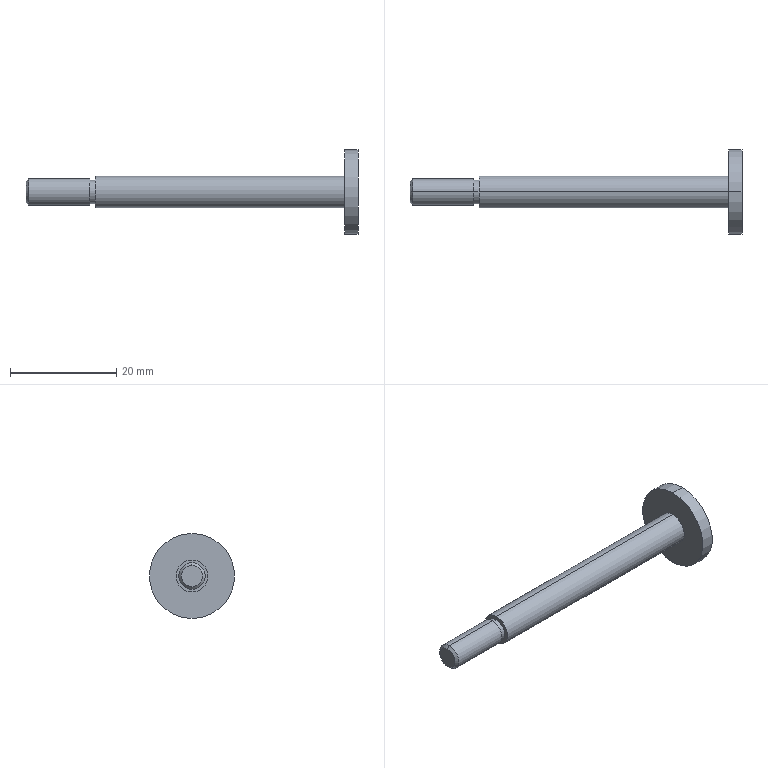Part | SolidWorks | features RefAxis 9, 3DProfileFeature 3, Revolution 3 | 1 solid | 15 faces | box 62.5 x 16 x 16 mm | volume 2081 mm3 | cylinder 8 | plane 5 | cone 2 | commonest cylinder face diameters 4.4 x2 5 x2 6 x2 16 x2
STEP:
#1=CARTESIAN_POINT('',(-23.509,0.,-2.5));
#2=VERTEX_POINT('',#1);
#3=CARTESIAN_POINT('',(-23.509,0.,2.5));
#4=VERTEX_POINT('',#3);
#5=CARTESIAN_POINT('',(-23.509,0.,0.));
#6=DIRECTION('',(1.,0.,0.));
#7=DIRECTION('',(0.,0.,-1.));
#8=AXIS2_PLACEMENT_3D('',#5,#6,#7);
#9=CIRCLE('',#8,2.5);
#10=EDGE_CURVE('',#2,#4,#9,.T.);
#11=ORIENTED_EDGE('',*,*,#10,.T.);
#12=CARTESIAN_POINT('',(-12.,0.,2.5));
#13=VERTEX_POINT('',#12);
#14=CARTESIAN_POINT('',(-12.,0.,2.5));
#15=DIRECTION('',(1.,0.,0.));
#16=VECTOR('',#15,1000.);
#17=LINE('',#14,#16);
#18=EDGE_CURVE('',#4,#13,#17,.T.);
#19=ORIENTED_EDGE('',*,*,#18,.T.);
#20=CARTESIAN_POINT('',(-12.,0.,-2.5));
#21=VERTEX_POINT('',#20);
#22=CARTESIAN_POINT('',(-12.,0.,0.));
#23=DIRECTION('',(1.,0.,0.));
#24=DIRECTION('',(0.,0.,-1.));
#25=AXIS2_PLACEMENT_3D('',#22,#23,#24);
#26=CIRCLE('',#25,2.5);
#27=EDGE_CURVE('',#21,#13,#26,.T.);
#28=ORIENTED_EDGE('',*,*,#27,.F.);
#29=CARTESIAN_POINT('',(-12.,0.,-2.5));
#30=DIRECTION('',(1.,0.,0.));
#31=VECTOR('',#30,1000.);
#32=LINE('',#29,#31);
#33=EDGE_CURVE('',#2,#21,#32,.T.);
#34=ORIENTED_EDGE('',*,*,#33,.F.);
#35=EDGE_LOOP('',(#11,#19,#28,#34));
#36=FACE_OUTER_BOUND('',#35,.T.);
#37=CARTESIAN_POINT('',(-12.,0.,0.));
#38=DIRECTION('',(1.,0.,0.));
#39=DIRECTION('',(0.,0.,-1.));
#40=AXIS2_PLACEMENT_3D('',#37,#38,#39);
#41=CYLINDRICAL_SURFACE('',#40,2.5);
#42=ADVANCED_FACE('',(#36),#41,.T.);
#43=CARTESIAN_POINT('',(-24.,0.,-2.01));
#44=VERTEX_POINT('',#43);
#45=CARTESIAN_POINT('',(-24.,0.,2.01));
#46=VERTEX_POINT('',#45);
#47=CARTESIAN_POINT('',(-24.,0.,0.));
#48=DIRECTION('',(1.,0.,0.));
#49=DIRECTION('',(0.,0.,-1.));
#50=AXIS2_PLACEMENT_3D('',#47,#48,#49);
#51=CIRCLE('',#50,2.01);
#52=EDGE_CURVE('',#44,#46,#51,.T.);
#53=ORIENTED_EDGE('',*,*,#52,.T.);
#54=CARTESIAN_POINT('',(-23.509,0.,2.5));
#55=DIRECTION('',(0.7071,0.,0.7071));
#56=VECTOR('',#55,1000.);
#57=LINE('',#54,#56);
#58=EDGE_CURVE('',#46,#4,#57,.T.);
#59=ORIENTED_EDGE('',*,*,#58,.T.);
#60=ORIENTED_EDGE('',*,*,#10,.F.);
#61=CARTESIAN_POINT('',(-23.509,0.,-2.5));
#62=DIRECTION('',(0.7071,0.,-0.7071));
#63=VECTOR('',#62,1000.);
#64=LINE('',#61,#63);
#65=EDGE_CURVE('',#44,#2,#64,.T.);
#66=ORIENTED_EDGE('',*,*,#65,.F.);
#67=EDGE_LOOP('',(#53,#59,#60,#66));
#68=FACE_OUTER_BOUND('',#67,.T.);
#69=CARTESIAN_POINT('',(-23.509,0.,0.));
#70=DIRECTION('',(1.,0.,0.));
#71=DIRECTION('',(0.,0.,-1.));
#72=AXIS2_PLACEMENT_3D('',#69,#70,#71);
#73=CONICAL_SURFACE('',#72,2.5,0.7854);
#74=ADVANCED_FACE('',(#68),#73,.T.);
#75=CARTESIAN_POINT('',(-12.,0.,2.2));
#76=VERTEX_POINT('',#75);
#77=CARTESIAN_POINT('',(-12.,0.,-2.2));
#78=VERTEX_POINT('',#77);
#79=CARTESIAN_POINT('',(-12.,0.,0.));
#80=DIRECTION('',(-1.,0.,0.));
#81=DIRECTION('',(0.,0.,-1.));
#82=AXIS2_PLACEMENT_3D('',#79,#80,#81);
#83=CIRCLE('',#82,2.2);
#84=EDGE_CURVE('',#76,#78,#83,.T.);
#85=ORIENTED_EDGE('',*,*,#84,.F.);
#86=CARTESIAN_POINT('',(-11.,0.,2.2));
#87=VERTEX_POINT('',#86);
#88=CARTESIAN_POINT('',(-11.,0.,2.2));
#89=DIRECTION('',(1.,0.,0.));
#90=VECTOR('',#89,1000.);
#91=LINE('',#88,#90);
#92=EDGE_CURVE('',#76,#87,#91,.T.);
#93=ORIENTED_EDGE('',*,*,#92,.T.);
#94=CARTESIAN_POINT('',(-11.,0.,-2.2));
#95=VERTEX_POINT('',#94);
#96=CARTESIAN_POINT('',(-11.,0.,0.));
#97=DIRECTION('',(-1.,0.,0.));
#98=DIRECTION('',(0.,0.,1.));
#99=AXIS2_PLACEMENT_3D('',#96,#97,#98);
#100=CIRCLE('',#99,2.2);
#101=EDGE_CURVE('',#87,#95,#100,.T.);
#102=ORIENTED_EDGE('',*,*,#101,.T.);
#103=CARTESIAN_POINT('',(-11.,0.,-2.2));
#104=DIRECTION('',(1.,0.,0.));
#105=VECTOR('',#104,1000.);
#106=LINE('',#103,#105);
#107=EDGE_CURVE('',#78,#95,#106,.T.);
#108=ORIENTED_EDGE('',*,*,#107,.F.);
#109=EDGE_LOOP('',(#85,#93,#102,#108));
#110=FACE_OUTER_BOUND('',#109,.T.);
#111=CARTESIAN_POINT('',(-11.,0.,0.));
#112=DIRECTION('',(1.,0.,0.));
#113=DIRECTION('',(0.,0.,-1.));
#114=AXIS2_PLACEMENT_3D('',#111,#112,#113);
#115=CYLINDRICAL_SURFACE('',#114,2.2);
#116=ADVANCED_FACE('',(#110),#115,.T.);
#117=CARTESIAN_POINT('',(36.,0.,-8.));
#118=VERTEX_POINT('',#117);
#119=CARTESIAN_POINT('',(36.,0.,8.));
#120=VERTEX_POINT('',#119);
#121=CARTESIAN_POINT('',(36.,0.,0.));
#122=DIRECTION('',(1.,0.,0.));
#123=DIRECTION('',(0.,0.,-1.));
#124=AXIS2_PLACEMENT_3D('',#121,#122,#123);
#125=CIRCLE('',#124,8.);
#126=EDGE_CURVE('',#118,#120,#125,.T.);
#127=ORIENTED_EDGE('',*,*,#126,.T.);
#128=CARTESIAN_POINT('',(38.5,0.,8.));
#129=VERTEX_POINT('',#128);
#130=CARTESIAN_POINT('',(38.5,0.,8.));
#131=DIRECTION('',(1.,0.,0.));
#132=VECTOR('',#131,1000.);
#133=LINE('',#130,#132);
#134=EDGE_CURVE('',#120,#129,#133,.T.);
#135=ORIENTED_EDGE('',*,*,#134,.T.);
#136=CARTESIAN_POINT('',(38.5,0.,-8.));
#137=VERTEX_POINT('',#136);
#138=CARTESIAN_POINT('',(38.5,0.,0.));
#139=DIRECTION('',(1.,0.,0.));
#140=DIRECTION('',(0.,0.,-1.));
#141=AXIS2_PLACEMENT_3D('',#138,#139,#140);
#142=CIRCLE('',#141,8.);
#143=EDGE_CURVE('',#137,#129,#142,.T.);
#144=ORIENTED_EDGE('',*,*,#143,.F.);
#145=CARTESIAN_POINT('',(38.5,0.,-8.));
#146=DIRECTION('',(1.,0.,0.));
#147=VECTOR('',#146,1000.);
#148=LINE('',#145,#147);
#149=EDGE_CURVE('',#118,#137,#148,.T.);
#150=ORIENTED_EDGE('',*,*,#149,.F.);
#151=EDGE_LOOP('',(#127,#135,#144,#150));
#152=FACE_OUTER_BOUND('',#151,.T.);
#153=CARTESIAN_POINT('',(38.5,0.,0.));
#154=DIRECTION('',(1.,0.,0.));
#155=DIRECTION('',(0.,0.,-1.));
#156=AXIS2_PLACEMENT_3D('',#153,#154,#155);
#157=CYLINDRICAL_SURFACE('',#156,8.);
#158=ADVANCED_FACE('',(#152),#157,.T.);
#159=CARTESIAN_POINT('',(-11.,0.,-3.));
#160=VERTEX_POINT('',#159);
#161=CARTESIAN_POINT('',(-11.,0.,3.));
#162=VERTEX_POINT('',#161);
#163=CARTESIAN_POINT('',(-11.,0.,0.));
#164=DIRECTION('',(1.,0.,0.));
#165=DIRECTION('',(0.,0.,-1.));
#166=AXIS2_PLACEMENT_3D('',#163,#164,#165);
#167=CIRCLE('',#166,3.);
#168=EDGE_CURVE('',#160,#162,#167,.T.);
#169=ORIENTED_EDGE('',*,*,#168,.T.);
#170=CARTESIAN_POINT('',(36.,0.,3.));
#171=VERTEX_POINT('',#170);
#172=CARTESIAN_POINT('',(38.5,0.,3.));
#173=DIRECTION('',(1.,0.,0.));
#174=VECTOR('',#173,1000.);
#175=LINE('',#172,#174);
#176=EDGE_CURVE('',#162,#171,#175,.T.);
#177=ORIENTED_EDGE('',*,*,#176,.T.);
#178=CARTESIAN_POINT('',(36.,0.,-3.));
#179=VERTEX_POINT('',#178);
#180=CARTESIAN_POINT('',(36.,0.,0.));
#181=DIRECTION('',(1.,0.,0.));
#182=DIRECTION('',(0.,0.,-1.));
#183=AXIS2_PLACEMENT_3D('',#180,#181,#182);
#184=CIRCLE('',#183,3.);
#185=EDGE_CURVE('',#179,#171,#184,.T.);
#186=ORIENTED_EDGE('',*,*,#185,.F.);
#187=CARTESIAN_POINT('',(38.5,0.,-3.));
#188=DIRECTION('',(1.,0.,0.));
#189=VECTOR('',#188,1000.);
#190=LINE('',#187,#189);
#191=EDGE_CURVE('',#160,#179,#190,.T.);
#192=ORIENTED_EDGE('',*,*,#191,.F.);
#193=EDGE_LOOP('',(#169,#177,#186,#192));
#194=FACE_OUTER_BOUND('',#193,.T.);
#195=CARTESIAN_POINT('',(38.5,0.,0.));
#196=DIRECTION('',(1.,0.,0.));
#197=DIRECTION('',(0.,0.,-1.));
#198=AXIS2_PLACEMENT_3D('',#195,#196,#197);
#199=CYLINDRICAL_SURFACE('',#198,3.);
#200=ADVANCED_FACE('',(#194),#199,.T.);
#201=CARTESIAN_POINT('',(-11.,0.,0.));
#202=DIRECTION('',(-1.,0.,0.));
#203=DIRECTION('',(0.,0.,1.));
#204=AXIS2_PLACEMENT_3D('',#201,#202,#203);
#205=CIRCLE('',#204,2.2);
#206=EDGE_CURVE('',#95,#87,#205,.T.);
#207=ORIENTED_EDGE('',*,*,#206,.F.);
#208=ORIENTED_EDGE('',*,*,#101,.F.);
#209=EDGE_LOOP('',(#207,#208));
#210=FACE_BOUND('',#209,.T.);
#211=ORIENTED_EDGE('',*,*,#168,.F.);
#212=CARTESIAN_POINT('',(-11.,0.,0.));
#213=DIRECTION('',(1.,0.,0.));
#214=DIRECTION('',(0.,0.,-1.));
#215=AXIS2_PLACEMENT_3D('',#212,#213,#214);
#216=CIRCLE('',#215,3.);
#217=EDGE_CURVE('',#162,#160,#216,.T.);
#218=ORIENTED_EDGE('',*,*,#217,.F.);
#219=EDGE_LOOP('',(#211,#218));
#220=FACE_OUTER_BOUND('',#219,.T.);
#221=CARTESIAN_POINT('',(-11.,0.,0.));
#222=DIRECTION('',(-1.,0.,0.));
#223=DIRECTION('',(0.,0.,1.));
#224=AXIS2_PLACEMENT_3D('',#221,#222,#223);
#225=PLANE('',#224);
#226=ADVANCED_FACE('',(#210,#220),#225,.T.);
#227=ORIENTED_EDGE('',*,*,#176,.F.);
#228=ORIENTED_EDGE('',*,*,#217,.T.);
#229=ORIENTED_EDGE('',*,*,#191,.T.);
#230=CARTESIAN_POINT('',(36.,0.,0.));
#231=DIRECTION('',(1.,0.,0.));
#232=DIRECTION('',(0.,0.,-1.));
#233=AXIS2_PLACEMENT_3D('',#230,#231,#232);
#234=CIRCLE('',#233,3.);
#235=EDGE_CURVE('',#171,#179,#234,.T.);
#236=ORIENTED_EDGE('',*,*,#235,.F.);
#237=EDGE_LOOP('',(#227,#228,#229,#236));
#238=FACE_OUTER_BOUND('',#237,.T.);
#239=CARTESIAN_POINT('',(38.5,0.,0.));
#240=DIRECTION('',(1.,0.,0.));
#241=DIRECTION('',(0.,0.,-1.));
#242=AXIS2_PLACEMENT_3D('',#239,#240,#241);
#243=CYLINDRICAL_SURFACE('',#242,3.);
#244=ADVANCED_FACE('',(#238),#243,.T.);
#245=ORIENTED_EDGE('',*,*,#185,.T.);
#246=ORIENTED_EDGE('',*,*,#235,.T.);
#247=EDGE_LOOP('',(#245,#246));
#248=FACE_BOUND('',#247,.T.);
#249=ORIENTED_EDGE('',*,*,#126,.F.);
#250=CARTESIAN_POINT('',(36.,0.,0.));
#251=DIRECTION('',(1.,0.,0.));
#252=DIRECTION('',(0.,0.,-1.));
#253=AXIS2_PLACEMENT_3D('',#250,#251,#252);
#254=CIRCLE('',#253,8.);
#255=EDGE_CURVE('',#120,#118,#254,.T.);
#256=ORIENTED_EDGE('',*,*,#255,.F.);
#257=EDGE_LOOP('',(#249,#256));
#258=FACE_OUTER_BOUND('',#257,.T.);
#259=CARTESIAN_POINT('',(36.,3.,0.));
#260=DIRECTION('',(-1.,0.,0.));
#261=DIRECTION('',(0.,0.,1.));
#262=AXIS2_PLACEMENT_3D('',#259,#260,#261);
#263=PLANE('',#262);
#264=ADVANCED_FACE('',(#248,#258),#263,.T.);
#265=ORIENTED_EDGE('',*,*,#134,.F.);
#266=ORIENTED_EDGE('',*,*,#255,.T.);
#267=ORIENTED_EDGE('',*,*,#149,.T.);
#268=CARTESIAN_POINT('',(38.5,0.,0.));
#269=DIRECTION('',(1.,0.,0.));
#270=DIRECTION('',(0.,0.,-1.));
#271=AXIS2_PLACEMENT_3D('',#268,#269,#270);
#272=CIRCLE('',#271,8.);
#273=EDGE_CURVE('',#129,#137,#272,.T.);
#274=ORIENTED_EDGE('',*,*,#273,.F.);
#275=EDGE_LOOP('',(#265,#266,#267,#274));
#276=FACE_OUTER_BOUND('',#275,.T.);
#277=CARTESIAN_POINT('',(38.5,0.,0.));
#278=DIRECTION('',(1.,0.,0.));
#279=DIRECTION('',(0.,0.,-1.));
#280=AXIS2_PLACEMENT_3D('',#277,#278,#279);
#281=CYLINDRICAL_SURFACE('',#280,8.);
#282=ADVANCED_FACE('',(#276),#281,.T.);
#283=ORIENTED_EDGE('',*,*,#143,.T.);
#284=ORIENTED_EDGE('',*,*,#273,.T.);
#285=EDGE_LOOP('',(#283,#284));
#286=FACE_OUTER_BOUND('',#285,.T.);
#287=CARTESIAN_POINT('',(38.5,8.,0.));
#288=DIRECTION('',(1.,0.,0.));
#289=DIRECTION('',(0.,0.,-1.));
#290=AXIS2_PLACEMENT_3D('',#287,#288,#289);
#291=PLANE('',#290);
#292=ADVANCED_FACE('',(#286),#291,.T.);
#293=ORIENTED_EDGE('',*,*,#92,.F.);
#294=CARTESIAN_POINT('',(-12.,0.,0.));
#295=DIRECTION('',(-1.,0.,0.));
#296=DIRECTION('',(0.,0.,-1.));
#297=AXIS2_PLACEMENT_3D('',#294,#295,#296);
#298=CIRCLE('',#297,2.2);
#299=EDGE_CURVE('',#78,#76,#298,.T.);
#300=ORIENTED_EDGE('',*,*,#299,.F.);
#301=ORIENTED_EDGE('',*,*,#107,.T.);
#302=ORIENTED_EDGE('',*,*,#206,.T.);
#303=EDGE_LOOP('',(#293,#300,#301,#302));
#304=FACE_OUTER_BOUND('',#303,.T.);
#305=CARTESIAN_POINT('',(-11.,0.,0.));
#306=DIRECTION('',(1.,0.,0.));
#307=DIRECTION('',(0.,0.,-1.));
#308=AXIS2_PLACEMENT_3D('',#305,#306,#307);
#309=CYLINDRICAL_SURFACE('',#308,2.2);
#310=ADVANCED_FACE('',(#304),#309,.T.);
#311=ORIENTED_EDGE('',*,*,#52,.F.);
#312=CARTESIAN_POINT('',(-24.,0.,0.));
#313=DIRECTION('',(1.,0.,0.));
#314=DIRECTION('',(0.,0.,-1.));
#315=AXIS2_PLACEMENT_3D('',#312,#313,#314);
#316=CIRCLE('',#315,2.01);
#317=EDGE_CURVE('',#46,#44,#316,.T.);
#318=ORIENTED_EDGE('',*,*,#317,.F.);
#319=EDGE_LOOP('',(#311,#318));
#320=FACE_OUTER_BOUND('',#319,.T.);
#321=CARTESIAN_POINT('',(-24.,0.,0.));
#322=DIRECTION('',(-1.,0.,0.));
#323=DIRECTION('',(0.,0.,1.));
#324=AXIS2_PLACEMENT_3D('',#321,#322,#323);
#325=PLANE('',#324);
#326=ADVANCED_FACE('',(#320),#325,.T.);
#327=ORIENTED_EDGE('',*,*,#58,.F.);
#328=ORIENTED_EDGE('',*,*,#317,.T.);
#329=ORIENTED_EDGE('',*,*,#65,.T.);
#330=CARTESIAN_POINT('',(-23.509,0.,0.));
#331=DIRECTION('',(1.,0.,0.));
#332=DIRECTION('',(0.,0.,-1.));
#333=AXIS2_PLACEMENT_3D('',#330,#331,#332);
#334=CIRCLE('',#333,2.5);
#335=EDGE_CURVE('',#4,#2,#334,.T.);
#336=ORIENTED_EDGE('',*,*,#335,.F.);
#337=EDGE_LOOP('',(#327,#328,#329,#336));
#338=FACE_OUTER_BOUND('',#337,.T.);
#339=CARTESIAN_POINT('',(-23.509,0.,0.));
#340=DIRECTION('',(1.,0.,0.));
#341=DIRECTION('',(0.,0.,-1.));
#342=AXIS2_PLACEMENT_3D('',#339,#340,#341);
#343=CONICAL_SURFACE('',#342,2.5,0.7854);
#344=ADVANCED_FACE('',(#338),#343,.T.);
#345=ORIENTED_EDGE('',*,*,#18,.F.);
#346=ORIENTED_EDGE('',*,*,#335,.T.);
#347=ORIENTED_EDGE('',*,*,#33,.T.);
#348=CARTESIAN_POINT('',(-12.,0.,0.));
#349=DIRECTION('',(1.,0.,0.));
#350=DIRECTION('',(0.,0.,-1.));
#351=AXIS2_PLACEMENT_3D('',#348,#349,#350);
#352=CIRCLE('',#351,2.5);
#353=EDGE_CURVE('',#13,#21,#352,.T.);
#354=ORIENTED_EDGE('',*,*,#353,.F.);
#355=EDGE_LOOP('',(#345,#346,#347,#354));
#356=FACE_OUTER_BOUND('',#355,.T.);
#357=CARTESIAN_POINT('',(-12.,0.,0.));
#358=DIRECTION('',(1.,0.,0.));
#359=DIRECTION('',(0.,0.,-1.));
#360=AXIS2_PLACEMENT_3D('',#357,#358,#359);
#361=CYLINDRICAL_SURFACE('',#360,2.5);
#362=ADVANCED_FACE('',(#356),#361,.T.);
#363=ORIENTED_EDGE('',*,*,#299,.T.);
#364=ORIENTED_EDGE('',*,*,#84,.T.);
#365=EDGE_LOOP('',(#363,#364));
#366=FACE_BOUND('',#365,.T.);
#367=ORIENTED_EDGE('',*,*,#27,.T.);
#368=ORIENTED_EDGE('',*,*,#353,.T.);
#369=EDGE_LOOP('',(#367,#368));
#370=FACE_OUTER_BOUND('',#369,.T.);
#371=CARTESIAN_POINT('',(-12.,2.5,0.));
#372=DIRECTION('',(1.,0.,0.));
#373=DIRECTION('',(0.,0.,-1.));
#374=AXIS2_PLACEMENT_3D('',#371,#372,#373);
#375=PLANE('',#374);
#376=ADVANCED_FACE('',(#366,#370),#375,.T.);
#377=CLOSED_SHELL('',(#42,#74,#116,#158,#200,#226,#244,#264,#282,#292,#310,#326,#344,#362,#376));
#378=MANIFOLD_SOLID_BREP('',#377);
#379=CARTESIAN_POINT('',(0.,0.,0.));
#380=DIRECTION('',(0.,0.,1.));
#381=DIRECTION('',(1.,0.,0.));
#382=AXIS2_PLACEMENT_3D('',#379,#380,#381);
#383=(LENGTH_UNIT()NAMED_UNIT(*)SI_UNIT(.MILLI.,.METRE.));
#384=UNCERTAINTY_MEASURE_WITH_UNIT(LENGTH_MEASURE(0.00001),#383,'','');
#385=(NAMED_UNIT(*)PLANE_ANGLE_UNIT()SI_UNIT($,.RADIAN.));
#386=(NAMED_UNIT(*)SI_UNIT($,.STERADIAN.)SOLID_ANGLE_UNIT());
#387=(GEOMETRIC_REPRESENTATION_CONTEXT(3)GLOBAL_UNCERTAINTY_ASSIGNED_CONTEXT((#384))GLOBAL_UNIT_ASSIGNED_CONTEXT((#383,#385,#386))REPRESENTATION_CONTEXT('',''));
#388=ADVANCED_BREP_SHAPE_REPRESENTATION('',(#378,#382),#387);